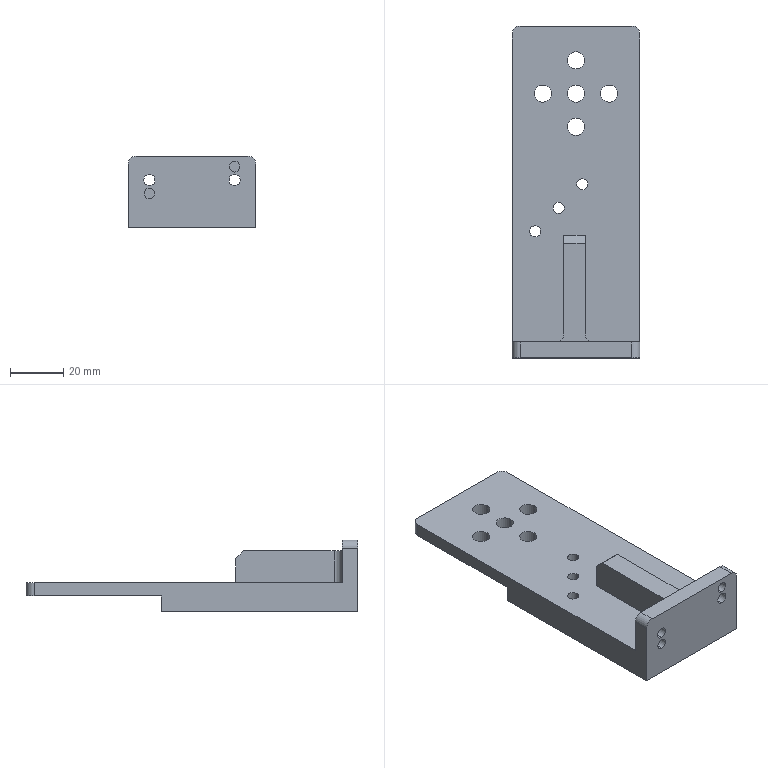NC program | NX | posted with a generic post | part box 48 x 124.7 x 27 mm
Whole program, first 1584 of 1777 lines:
N10 G17 G21 G94 G90
(FLOOR_WALL_COPY , TOOL : D80)
N12 T19 M6
N14 G54
N16 G17 G0 G90 X-111.35 Y0. B0. C0. S6500 M3
N18 G43 Z30. H19
N20 Z3.
N22 G94 G1 Z0. F1500.
N24 X-106.35
N26 X106.35
N28 X111.35
N30 Z3.
N32 G0 Z30.
N34 M5
(ADAPTIVE_MILLING , TOOL : D10)
N36 T15 M6
N38 G54
N40 G17 G0 G90 X-0.035 Y35.706 B0. C0. S9500 M3
N42 G43 Z30. H15
N44 Z-2.85
N46 G94 G1 Z-5.85 F1000.
N48 X-0.314 Y34.925 F3000.
N50 X-0.57 Y34.137
N52 G3 X-0.035 Y33.059 R1.017
N54 X3.029 Y32.298 R8.28
N56 X12.896 Y32.015 R111.643
N58 G1 X15.146 Y32.011
N60 X19.021 Y32.008
N62 X32.646 Y32.007
N64 X63.271
N66 X63.396 Y32.006
N68 X63.521 Y32.004
N70 G2 X67.796 Y29.5 R5.713
N72 X69.831 Y24.05 R12.236
N74 X70.306 Y15.57 R62.176
N76 G1 X70.315 Y14.446
N78 X70.323 Y13.071
N80 X70.329 Y11.196
N82 X70.333 Y8.446
N84 X70.335 Y3.071
N86 X70.336 Y-25.054
N88 G2 X67.993 Y-29.286 R5.635
N90 X62.588 Y-31.431 R11.953
N92 X54.988 Y-31.94 R51.981
N94 G1 X53.988 Y-31.953
N96 X52.988 Y-31.962
N98 X51.613 Y-31.971
N100 X49.863 Y-31.977
N102 X47.238 Y-31.982
N104 X42.613 Y-31.984
N106 X3.363 Y-31.985
N108 X-63.387
N110 X-63.512 Y-31.983
N112 X-63.637 Y-31.976
N114 X-63.762 Y-31.965
N116 G2 X-67.992 Y-29.146 R6.011
N118 X-69.896 Y-23.51 R13.346
N120 X-70.314 Y-14.526 R75.467
N122 G1 X-70.322 Y-13.151
N124 X-70.329 Y-11.276
N126 X-70.333 Y-8.651
N128 X-70.335 Y-3.651
N130 X-70.336 Y24.974
N132 X-70.335 Y25.099
N134 G2 X-67.854 Y29.389 R5.736
N136 X-62.294 Y31.479 R12.387
N138 X-53.814 Y31.955 R61.959
N140 G1 X-52.689 Y31.964
N142 X-51.314 Y31.972
N144 X-49.439 Y31.978
N146 X-46.689 Y31.983
N148 X-41.314 Y31.985
N150 X-3.814
N152 G2 X1.658 Y31.464 R60.908
N154 G3 X13.521 Y31.035 R127.721
N156 G1 X15.146 Y31.028
N158 X17.521 Y31.023
N160 X21.146 Y31.019
N162 X29.521 Y31.018
N164 X60.271 Y31.017
N166 X60.521 Y31.013
N168 G2 X66.702 Y27.322 R7.626
N170 X68.839 Y20.846 R15.66
N172 X69.3 Y10.988 R84.585
N174 G1 X69.309 Y9.613
N176 X69.316 Y7.863
N178 X69.321 Y5.363
N180 X69.324 Y1.238
N182 X69.325 Y-12.137
N184 Y-21.887
N186 G2 X65.75 Y-28.259 R7.595
N188 X59.299 Y-30.464 R15.393
N190 X49.942 Y-30.943 R76.184
N192 G1 X48.693 Y-30.953
N194 X47.193 Y-30.961
N196 X45.193 Y-30.967
N198 X42.318 Y-30.972
N200 X36.818 Y-30.974
N202 X-60.182
N204 X-60.432 Y-30.972
N206 X-60.682 Y-30.963
N208 X-60.807 Y-30.955
N210 G2 X-66.715 Y-27.232 R7.692
N212 X-68.841 Y-20.752 R15.777
N214 X-69.3 Y-10.893 R83.753
N216 G1 X-69.309 Y-9.519
N218 X-69.316 Y-7.769
N220 X-69.321 Y-5.269
N222 X-69.324 Y-1.269
N224 X-69.325 Y11.606
N226 Y21.856
N228 G2 X-65.669 Y28.31 R7.607
N230 X-59.079 Y30.493 R15.728
N232 X-49.971 Y30.943 R78.281
N234 G1 X-48.846 Y30.952
N236 X-47.471 Y30.96
N238 X-45.596 Y30.966
N240 X-42.846 Y30.971
N242 X-37.971 Y30.974
N244 X-6.221
N246 G2 X1.386 Y30.485 R99.342
N248 G3 X16.375 Y30.042 R194.129
N250 G1 X18.75 Y30.035
N252 X22.125 Y30.031
N254 X28.375 Y30.029
N256 X57.25 Y30.028
N258 X57.75 Y30.026
N260 X57.875 Y30.024
N262 G2 X65.811 Y25.229 R8.947
N264 X67.86 Y18.194 R18.674
N266 X68.285 Y8.458 R94.495
N268 G1 X68.294 Y7.083
N270 X68.302 Y5.333
N272 X68.309 Y2.833
N274 X68.312 Y-0.542
N276 X68.314 Y-8.042
N278 Y-19.292
N280 G2 X63.502 Y-27.467 R8.952
N282 X56.466 Y-29.51 R18.542
N284 X44.98 Y-29.945 R112.673
N286 G1 X43.105 Y-29.953
N288 X40.73 Y-29.958
N290 X36.855 Y-29.962
N292 X27.605 Y-29.964
N294 X-57.645
N296 X-57.895 Y-29.961
N298 G2 X-61.662 Y-29.177 R9.459
N300 X-63.747 Y-28.948 R16.345
N302 X-66.837 Y-26.511 R5.458
N304 X-67.495 Y-24.034 R5.984
N306 X-68.289 Y-8.94 R124.153
N308 G1 X-68.297 Y-7.44
N310 X-68.304 Y-5.565
N312 X-68.309 Y-2.94
N314 X-68.313 Y1.06
N316 X-68.314 Y11.185
N318 Y19.31
N320 G2 X-67.526 Y23.327 R9.637
N322 X-67.298 Y25.397 R15.666
N324 X-64.861 Y28.487 R5.458
N326 X-62.384 Y29.145 R5.984
N328 X-47.79 Y29.934 R121.449
N330 G1 X-46.29 Y29.944
N332 X-44.415 Y29.952
N334 X-42.04 Y29.957
N336 X-38.415 Y29.961
N338 X-30.915 Y29.963
N340 X-7.915 Y29.964
N342 G2 X0.822 Y29.518 R127.25
N344 G3 X12.709 Y29.114 R215.245
N346 X27.959 Y29.04 R784.32
N348 G1 X43.084 Y29.039
N350 X54.334
N352 X55.084 Y29.034
N354 X55.584 Y29.029
N356 X55.834 Y29.024
N358 X56.083 Y29.016
N360 G2 X64.76 Y23.61 R9.841
N362 X66.811 Y16.443 R19.883
N364 X67.27 Y6.208 R98.656
N366 G1 X67.281 Y4.833
N368 X67.289 Y3.208
N370 X67.295 Y1.083
N372 X67.3 Y-1.792
N374 X67.303 Y-6.917
N376 X67.304 Y-16.917
N378 G2 X65.585 Y-23.196 R10.36
N380 X59.426 Y-27.465 R11.896
N382 X51.799 Y-28.717 R30.693
N384 X38.178 Y-28.947 R261.114
N386 G1 X34.428 Y-28.951
N388 X26.178 Y-28.953
N390 X13.053
N392 X12.928 Y-28.959
N394 X12.887 Y-28.964
N396 X12.814 Y-28.984
N398 X11.584 Y-29.145
N400 X11.515 Y-29.15
N402 X-61.86
N404 G2 X-64.98 Y-28.418 R6.001
N406 X-67.334 Y-25.264 R5.458
N408 G1 X-67.495 Y-24.034
N410 X-67.5 Y-23.965
N412 Y23.535
N414 G2 X-66.768 Y26.63 R5.985
N416 X-63.614 Y28.984 R5.458
N418 G1 X-62.384 Y29.145
N420 X-62.315 Y29.15
N422 X11.515
N424 X11.584 Y29.145
N426 G2 X13.901 Y28.652 R9.504
N428 G3 X20.119 Y28.12 R34.015
N430 X35.869 Y28.05 R800.024
N432 G2 X54.493 Y28.002 R972.856
N434 X63.712 Y22.117 R10.517
N436 X65.769 Y14.819 R20.994
N438 X66.261 Y3.586 R105.233
N440 X66.256 Y-16.289 R937.524
N442 X60.371 Y-25.373 R10.478
N444 X53.193 Y-27.402 R21.037
N446 X41.71 Y-27.913 R104.229
N448 G1 X40.21 Y-27.922
N450 X38.335 Y-27.93
N452 X35.835 Y-27.936
N454 X32.085 Y-27.94
N456 X24.335 Y-27.942
N458 X16.085
N460 G3 X14.723 Y-28.044 R4.18
N462 G2 X12.827 Y-28.98 R6.626
N464 G3 X12.244 Y-30.51 R1.013
N466 G1 X12.605 Y-31.07
N468 X12.988 Y-31.616
N470 G3 X14.734 Y-30.901 R1.011
N472 G1 Z-2.85
N474 G0 Z30.
N476 X13.274 Y31.436
N478 Z-2.85
N480 G1 Z-5.85 F1000.
N482 G3 X11.457 Y30.806 R-1.01 F3000.
N484 G1 X12.729 Y29.125
N486 X12.887 Y28.999
N488 X13.063 Y28.9
N490 G3 X15.214 Y27.979 R69.717
N492 X20.897 Y27.212 R23.518
N494 X35.646 Y27.062 R427.881
N496 G2 X52.895 Y26.992 R751.352
N498 X62.736 Y20.577 R11.125
N500 X64.781 Y12.887 R22.827
N502 X65.251 Y1.526 R117.565
N504 X65.247 Y-14.473 R800.273
N506 X58.794 Y-24.409 R11.075
N508 X50.973 Y-26.45 R23.107
N510 X39.237 Y-26.904 R123.61
N512 G1 X37.612 Y-26.913
N514 X35.612 Y-26.92
N516 X32.612 Y-26.926
N518 X28.487 Y-26.93
N520 X18.987 Y-26.931
N522 X18.112 Y-26.937
N524 G3 X15.755 Y-27.138 R8.582
N526 X15.136 Y-27.684 R2.117
N528 G1 X14.541 Y-28.141
N530 G3 X14.489 Y-29.7 R1.013
N532 G1 X14.885 Y-30.052
N534 X15.294 Y-30.389
N536 G3 X16.836 Y-29.501 R1.012
N538 G1 Z-2.85
N540 G0 Z30.
N542 X15.049 Y30.779
N544 Z-2.85
N546 G1 Z-5.85 F1000.
N548 G3 X13.134 Y30.302 R-1.01 F3000.
N550 G1 X13.54 Y29.465
N552 X13.968 Y28.639
N554 X14.18 Y28.418
N556 G3 X17.78 Y26.79 R7.326
N558 X25.618 Y26.149 R46.049
N560 X45.743 Y26.069 R974.003
N562 G2 X52.363 Y25.901 R79.379
N564 X61.578 Y19.463 R11.462
N566 X63.735 Y11.546 R22.992
N568 X64.235 Y0.063 R114.775
N570 X64.22 Y-13.062 R417.223
N572 X57.455 Y-23.362 R11.529
N574 X49.509 Y-25.42 R23.817
N576 X37.274 Y-25.893 R127.791
N578 G1 X35.899 Y-25.901
N580 X33.899 Y-25.909
N582 X31.149 Y-25.915
N584 X27.024 Y-25.919
N586 X22.024 Y-25.92
N588 X20.899 Y-25.927
N590 X19.649 Y-25.937
N592 X19.274 Y-25.943
N594 X19.149 Y-25.946
N596 G3 X16.317 Y-26.336 R8.21
N598 G1 X16.211 Y-26.401
N600 X16.112 Y-26.478
N602 X16.02 Y-26.563
N604 X15.996 Y-26.58
N606 X15.968 Y-26.63
N608 X15.359 Y-27.424
N610 G3 X15.286 Y-28.532 R1.01
N612 X16.044 Y-29.031 Z-5.803 R1.046
N614 G1 X17.082 Y-29.246 Z-5.75
N616 X19.154 Y-29.668
N618 X33.631 Y-29.674
N620 G3 X47.321 Y-28.765 R104.449
N622 G1 X49.901 Y-28.424
N624 X52.478 Y-28.063
N626 G3 X59.478 Y-25.702 R23.042
N628 X62.152 Y-24.032 R32.386
N630 X63.976 Y-22.197 R8.956
N632 X66.464 Y-17.488 R16.584
N634 X66.915 Y-15.424 R14.301
N636 X67.368 Y-11.085 R37.066
N638 X67.445 Y-6.096 R62.706
N640 G1 X67.07 Y8.277
N642 G3 X66.414 Y14.473 R39.88
N644 G1 X66.185 Y15.699
N646 X65.904 Y16.914
N648 G3 X64.777 Y19.798 R16.586
N650 X62.924 Y23.047 R22.
N652 X61.061 Y25.285 R29.178
N654 X59.448 Y26.546 R7.461
N656 X56.779 Y27.894 R27.167
N658 X54.264 Y28.577 R12.145
N660 X50.556 Y28.975 R22.955
N662 G1 X18.819 Y29.713
N664 X16.615 Y29.722
N666 X15.961 Y29.73 Z-5.783
N668 X15.308 Y29.713 Z-5.815
N670 G3 X14.717 Y29.379 Z-5.85 R1.038
N672 X14.492 Y28.548 R1.016
N674 X15.136 Y27.684 R1.295
N676 X17.835 Y26.169 R5.508
N678 X24.633 Y25.261 R29.771
N680 X42.381 Y25.083 R489.163
N682 G2 X50.503 Y24.933 R136.592
N684 X60.618 Y18.01 R11.9
N686 X62.729 Y9.949 R24.232
N688 X63.225 Y-1.91 R119.841
N690 X63.191 Y-11.784 R216.134
N692 X56.252 Y-22.275 R11.909
N694 X48.314 Y-24.367 R24.155
N696 X36.455 Y-24.876 R119.317
N698 G1 X34.955 Y-24.886
N700 X33.08 Y-24.894
N702 X30.705 Y-24.901
N704 X27.455 Y-24.906
N706 X24.955 Y-24.908
N708 X23.955 Y-24.915
N710 X23.205 Y-24.917
N712 X22.205 Y-24.923
N714 X21.33 Y-24.933
N716 X20.955 Y-24.938
N718 G3 X17.121 Y-25.38 R13.244
N720 X16.037 Y-26.511 R1.532
N722 G1 X15.974 Y-26.619
N724 G3 X15.97 Y-27.612 R1.014
N726 X16.696 Y-28.113 Z-5.805 R1.05
N728 G1 X17.753 Y-28.375 Z-5.75
N730 X19.75 Y-28.862
N732 X24.888 Y-28.873
N734 X30.025 Y-28.854
N736 G3 X44.191 Y-27.92 R140.231
N738 G1 X47.666 Y-27.517
N740 X51.139 Y-27.089
N742 G3 X57.523 Y-25.034 R21.966
N744 X62.06 Y-21.845 R15.427
N746 G1 X63.212 Y-20.641
N748 G3 X64.339 Y-18.926 R7.881
N750 X65.496 Y-16.169 R28.464
N752 X65.901 Y-14.227 R9.459
N754 X66.375 Y-8.003 R117.455
N756 G1 X66.512 Y-5.039
N758 X66.594 Y-2.073
N760 G3 X66.182 Y6.333 R74.972
N762 G1 X65.907 Y8.922
N764 X65.618 Y11.509
N766 G3 X64.747 Y15.568 R28.451
N768 G1 X64.394 Y16.765
N770 X63.997 Y17.95
N772 G3 X62.296 Y21.274 R16.442
N774 G1 X61.314 Y22.719
N776 G3 X57.949 Y25.628 R10.939
N778 X53.23 Y27.478 R14.704
N780 X50.274 Y27.879 R21.595
N782 G1 X19.131 Y29.836
N784 X18.861 Y29.817
N786 X16.97 Y29.417
N788 X16.314 Y29.283 Z-5.784
N790 X15.662 Y29.126 Z-5.817
N792 G3 X15.168 Y28.707 Z-5.85 R1.041
N794 X15.234 Y27.586 R1.01
N796 X18.221 Y25.446 R5.386
N798 X24.861 Y24.35 R26.004
N800 X39.482 Y24.098 R278.956
N802 G2 X48.854 Y23.949 R187.644
N804 X56.948 Y20.497 R12.355
N806 X60.906 Y13.091 R15.896
N808 X62.061 Y3.678 R46.236
N810 X62.172 Y-10.318 R212.705
N812 X58.773 Y-18.56 R12.342
N814 X51.623 Y-22.481 R15.607
N816 X42.72 Y-23.674 R42.357
N818 X25.098 Y-23.908 R462.336
N820 G3 X18.984 Y-24.169 R46.763
N822 X16.772 Y-24.956 R4.616
N824 X16.211 Y-26.09 R3.818
N826 X16.438 Y-27.19 R1.01
N828 X17.296 Y-27.464 Z-5.803 R1.047
N830 G1 X18.362 Y-27.395 Z-5.75
N832 X20.558 Y-27.255
N834 X36.808
N836 G3 X46.749 Y-26.495 R65.951
N838 G1 X50.575 Y-25.893
N840 G3 X57.678 Y-23.135 R20.586
N842 X60.422 Y-21.239 R29.156
N844 X62.956 Y-18.409 R13.153
N846 X64.481 Y-15.028 R10.236
N848 X65.036 Y-11.711 R25.141
N850 G1 X65.124 Y-10.592
N852 X65.171 Y-9.471
N854 X65.343 Y0.528
N856 G3 X64.752 Y9.227 R52.015
N858 G1 X64.246 Y12.435
N860 G3 X63.062 Y16.496 R20.997
N862 X61.92 Y18.704 R16.474
N864 G1 X60.264 Y21.343
N866 G3 X59.286 Y22.55 R7.279
N868 G1 X58.262 Y23.418
N870 X57.226 Y24.271
N872 G3 X54.4 Y25.83 R12.036
N874 X50.783 Y26.713 R12.454
N876 X42.684 Y27.242 R186.451
N878 G1 X19.95 Y28.163
N880 X17.747 Y28.446
N882 X17.095 Y28.535 Z-5.783
N884 X16.441 Y28.599 Z-5.816
N886 G3 X15.819 Y28.347 Z-5.85 R1.039
N888 X15.691 Y26.991 R1.005
N890 X17.102 Y25.471 R5.483
N892 X21.921 Y23.831 R12.773
N894 X31.89 Y23.172 R70.477
N896 G2 X46.888 Y22.988 R775.762
N898 X53.889 Y20.965 R13.899
N900 X59.182 Y14.034 R13.777
N902 X60.83 Y5.722 R31.255
N904 X61.135 Y-9.142 R141.978
N906 X57.546 Y-17.567 R12.593
N908 X50.368 Y-21.444 R16.016
N910 X41.341 Y-22.657 R42.942
N912 X24.72 Y-22.916 R482.485
N914 G3 X18.874 Y-23.372 R28.465
N916 X16.857 Y-24.309 R4.386
N918 X16.501 Y-25.385 R2.115
N920 X16.758 Y-26.348 R1.014
N922 X17.594 Y-26.64 Z-5.804 R1.049
N924 G1 X18.678 Y-26.61 Z-5.75
N926 X20.848 Y-26.549
N928 X30.223
N930 G3 X43.913 Y-25.641 R104.449
N932 G1 X46.7 Y-25.271
N934 X49.484 Y-24.887
N936 G3 X55.884 Y-22.536 R19.394
N938 X60.14 Y-19.304 R21.663
N940 X62.335 Y-16.003 R11.567
N942 G1 X63.337 Y-13.721
N944 G3 X63.827 Y-11.924 R6.864
N946 G1 X64.26 Y-7.753
N948 G3 X64.343 Y-1.346 R46.365
N950 G1 X64.108 Y2.814
N952 X63.852 Y6.972
N954 G3 X61.943 Y15.254 R32.188
N956 X59.611 Y19.643 R19.899
N958 X57.989 Y21.524 R15.572
N960 G1 X56.348 Y23.119
N962 G3 X53.266 Y24.853 R8.95
N964 X48.017 Y25.817 R23.24
N966 G1 X18.191 Y27.816
N968 X17.525 Y27.864 Z-5.783
N970 X16.859 Y27.888 Z-5.817
N972 G3 X16.266 Y27.613 Z-5.85 R1.04
N974 X16.037 Y26.511 R1.01
N976 X17.94 Y24.444 R3.889
N978 X23.412 Y22.786 R15.731
N980 X34.137 Y22.173 R85.721
N982 G2 X45.635 Y21.984 R484.936
N984 X52.646 Y19.977 R14.365
N986 X58.124 Y12.884 R13.949
N988 X59.82 Y4.328 R31.846
N990 X60.087 Y-8.036 R103.638
N992 X56.099 Y-16.795 R12.688
N994 X48.578 Y-20.56 R16.926
N996 X39.159 Y-21.679 R49.273
N998 X24.287 Y-21.938 R840.384
N1000 G3 X18.721 Y-22.625 R21.206
N1002 X16.825 Y-23.767 R3.615
N1004 X16.587 Y-24.857 R3.059
N1006 X16.955 Y-25.769 R1.014
N1008 X17.759 Y-25.99 Z-5.807 R1.173
N1010 G1 X18.905 Y-26.001 Z-5.75
N1012 X21.481 Y-26.012
N1014 X24.056 Y-25.965
N1016 G3 X30.289 Y-25.626 R89.658
N1018 G1 X44.607 Y-24.324
N1020 G3 X54.182 Y-21.719 R28.478
N1022 G1 X55.268 Y-21.206
N1024 X56.347 Y-20.677
N1026 G3 X59.221 Y-18.24 R9.631
N1028 X61.246 Y-15.105 R17.5
N1030 X62.769 Y-10.433 R14.094
N1032 X63.158 Y-5.465 R42.479
N1034 G1 X63.232 Y-0.604
N1036 G3 X62.425 Y8.208 R51.287
N1038 G1 X62.095 Y10.052
N1040 X61.747 Y11.893
N1042 G3 X60.067 Y16.16 R15.692
N1044 X58.85 Y18.041 R20.831
N1046 G1 X58.124 Y19.026
N1048 X57.362 Y19.983
N1050 G3 X55.375 Y21.853 R11.039
N1052 G1 X54.957 Y22.122
N1054 X54.529 Y22.373
N1056 X53.433 Y22.962
N1058 X52.316 Y23.512
N1060 G3 X49.252 Y24.485 R12.582
N1062 X38.826 Y25.648 R274.358
N1064 G1 X20.499 Y27.331
N1066 X18.358 Y27.468
N1068 X17.683 Y27.516 Z-5.784
N1070 X17.007 Y27.542 Z-5.818
N1072 G3 X16.427 Y27.283 Z-5.85 R1.042
N1074 X16.18 Y26.164 R1.01
N1076 X18.53 Y23.533 R4.519
N1078 X24.498 Y21.793 R17.436
N1080 X34.849 Y21.191 R89.248
N1082 G2 X44.845 Y20.951 R222.906
N1084 X52.406 Y18.316 R13.844
N1086 X57.312 Y11.077 R14.956
N1088 X58.873 Y2.112 R36.215
N1090 X59.014 Y-7.13 R69.228
N1092 X51.673 Y-17.98 R12.801
N1094 X43.145 Y-20.266 R25.644
N1096 X32.163 Y-20.812 R109.366
N1098 G3 X22.793 Y-21.065 R174.236
N1100 X18.065 Y-22.132 R13.322
N1102 X16.77 Y-23.256 R2.532
N1104 X16.679 Y-24.158 R4.534
N1106 X17.078 Y-25.094 R1.011
N1108 X17.856 Y-25.291 Z-5.809 R1.199
N1110 G1 X19.036 Y-25.304 Z-5.75
N1112 X21.026 Y-25.323
N1114 X38.474 Y-23.981
N1116 G3 X45.889 Y-22.952 R62.285
N1118 G1 X48.337 Y-22.447
N1120 G3 X52.128 Y-21.068 R18.9
N1122 X56.196 Y-18.768 R41.277
N1124 X57.41 Y-17.8 R6.639
N1126 X59.153 Y-15.603 R30.304
N1128 X61.526 Y-9.926 R14.502
N1130 G1 X61.836 Y-8.185
N1132 X62.106 Y-6.437
N1134 G3 X62.245 Y-3.119 R16.457
N1136 G1 X61.98 Y0.829
N1138 X61.69 Y4.776
N1140 G3 X60.831 Y9.896 R38.241
N1142 G1 X60.54 Y11.108
N1144 X60.195 Y12.306
N1146 G3 X58.429 Y15.853 R16.02
N1148 X56.345 Y18.647 R32.723
N1150 X49.749 Y23.07 R13.028
N1152 X46.702 Y23.69 R18.346
N1154 G1 X20.765 Y26.64
N1156 X18.653 Y26.775
N1158 X17.975 Y26.823 Z-5.784
N1160 X17.295 Y26.849 Z-5.818
N1162 G3 X16.72 Y26.595 Z-5.85 R1.043
N1164 X16.467 Y25.471 R1.007
N1166 X18.193 Y23.151 R3.804
N1168 X23.531 Y21.126 R14.162
N1170 X32.983 Y20.274 R60.021
N1172 G2 X43.353 Y19.978 R340.49
N1174 X50.774 Y17.648 R14.664
N1176 X56.142 Y10.304 R14.643
N1178 X57.797 Y1.611 R33.954
N1180 X57.879 Y-6.626 R44.639
N1182 X50.631 Y-16.883 R12.833
N1184 X42.613 Y-19.161 R24.921
N1186 X30.637 Y-19.812 R110.188
N1188 G3 X22.151 Y-20.223 R85.513
N1190 X17.76 Y-21.561 R11.098
N1192 X16.717 Y-22.75 R2.044
N1194 G1 X16.7 Y-22.872
N1196 Y-23.622
N1198 G3 X17.252 Y-24.516 R1.011
N1200 X18.18 Y-24.52 Z-5.802 R1.139
N1202 G1 X19.174 Y-24.209 Z-5.75
N1204 X20.108 Y-23.91
N1206 X21.049 Y-23.634
N1208 X21.2 Y-23.622
N1210 X27.627 Y-23.61
N1212 G3 X36.161 Y-23.002 R81.628
N1214 G1 X40.295 Y-22.49
N1216 X44.427 Y-21.957
N1218 G3 X53.607 Y-18.807 R27.116
N1220 X56.917 Y-16.05 R13.601
N1222 X60.261 Y-10.152 R14.873
N1224 X61.2 Y-3.738 R23.335
N1226 G1 Y-1.703
N1228 X61.143 Y0.33
N1230 G3 X59.441 Y9.938 R42.347
N1232 X57.462 Y14.485 R22.102
N1234 G1 X56.202 Y16.638
N1236 G3 X55.043 Y18.098 R7.28
N1238 X52.082 Y20.381 R15.814
N1240 X47.281 Y22.342 R15.328
N1242 X45.076 Y22.712 R20.646
N1244 G1 X20.921 Y25.282
N1246 X18.953 Y25.958
N1248 X18.326 Y26.181 Z-5.783
N1250 X17.691 Y26.381 Z-5.817
N1252 G3 X17.044 Y26.271 Z-5.85 R1.04
N1254 X16.534 Y25.264 R1.01
N1256 X17.868 Y22.813 R3.412
N1258 X22.438 Y20.586 R11.634
N1260 X31.466 Y19.39 R42.69
N1262 G2 X41.958 Y19.008 R855.284
N1264 X48.994 Y17.04 R15.649
N1266 X54.871 Y9.8 R14.315
N1268 X56.712 Y1.149 R31.295
N1270 X56.653 Y-6.455 R29.907
N1272 X49.619 Y-15.777 R12.854
N1274 X41.246 Y-18.157 R25.048
N1276 X32.019 Y-18.75 R94.343
N1278 G3 X23.157 Y-19.187 R108.754
N1280 X18.127 Y-20.573 R13.783
N1282 X16.771 Y-21.823 R3.031
N1284 X16.7 Y-22.997 R4.011
N1286 X17.264 Y-23.897 R1.011
N1288 X18.176 Y-23.897 Z-5.803 R1.149
N1290 G1 X19.19 Y-23.588 Z-5.75
N1292 X21.094 Y-23.012
N1294 X39.262 Y-21.492
N1296 G3 X45.418 Y-20.514 R42.568
N1298 G1 X46.632 Y-20.227
N1300 X47.834 Y-19.893
N1302 G3 X51.441 Y-18.236 R17.985
N1304 G1 X52.391 Y-17.642
N1306 X53.315 Y-17.009
N1308 X54.275 Y-16.315
N1310 X55.225 Y-15.606
N1312 G3 X57.152 Y-13.35 R8.994
N1314 X58.105 Y-11.464 R14.871
N1316 X59.781 Y-5.748 R23.1
N1318 X59.992 Y-0.534 R19.419
N1320 G1 X59.576 Y3.401
N1322 G3 X56.907 Y12.769 R33.913
N1324 X54.466 Y16.358 R12.938
N1326 G1 X52.771 Y18.069
N1328 G3 X50.158 Y19.852 R10.924
N1330 X46.696 Y21.233 R19.72
N1332 G1 X45.79 Y21.446
N1334 X44.872 Y21.604
N1336 X21.001 Y24.786
N1338 X19.041 Y25.456
N1340 X18.404 Y25.681 Z-5.784
N1342 X17.759 Y25.884 Z-5.818
N1344 G3 X17.13 Y25.787 Z-5.85 R1.042
N1346 X16.599 Y24.768 R1.007
N1348 X18.1 Y21.998 R3.773
N1350 X23.017 Y19.633 R12.605
N1352 X32.419 Y18.402 R45.593
N1354 G2 X41.283 Y17.985 R254.256
N1356 X48.973 Y15.303 R14.933
N1358 X54.078 Y8.052 R15.209
N1360 X55.671 Y-4.387 R31.712
N1362 X48.522 Y-14.715 R12.853
N1364 X40.157 Y-17.124 R24.935
N1366 X29.933 Y-17.789 R109.912
N1368 G3 X22.092 Y-18.443 R58.951
N1370 X17.571 Y-20.157 R10.962
N1372 X16.7 Y-21.354 R1.854
N1374 G1 Y-22.229
N1376 G3 X17.264 Y-23.129 R1.011
N1378 X18.176 Y-23.13 Z-5.803 R1.149
N1380 G1 X19.19 Y-22.821 Z-5.75
N1382 X21.098 Y-22.244
N1384 X36.138 Y-20.871
N1386 G3 X45.848 Y-19.056 R53.573
N1388 X51.082 Y-17.016 R35.109
N1390 X55.002 Y-13.829 R12.152
N1392 X57.573 Y-9.695 R18.953
N1394 X58.895 Y-3.76 R13.232
N1396 X58.479 Y2.67 R47.049
N1398 X57.69 Y6.749 R35.547
N1400 X54.722 Y13.517 R24.012
N1402 G1 X54.129 Y14.439
N1404 X53.499 Y15.336
N1406 G3 X50.56 Y17.99 R10.835
N1408 X46.086 Y20.127 R20.505
N1410 X41.29 Y21.315 R24.469
N1412 G1 X21.086 Y24.166
N1414 X19.131 Y24.834
N1416 X18.49 Y25.06 Z-5.784
N1418 X17.842 Y25.264 Z-5.818
N1420 G3 X17.22 Y25.171 Z-5.85 R1.043
N1422 X16.68 Y24.148 R1.007
N1424 X17.876 Y21.564 R3.486
N1426 X22.651 Y18.942 R11.633
N1428 X31.393 Y17.53 R38.723
N1430 G2 X40.376 Y16.989 R284.794
N1432 X48.019 Y14.18 R14.902
N1434 X53.11 Y6.766 R15.534
N1436 X54.475 Y-3.57 R25.362
N1438 X47.619 Y-13.552 R12.681
N1440 X39.534 Y-16.025 R24.039
N1442 X30.067 Y-16.763 R99.057
N1444 G3 X21.99 Y-17.573 R55.47
N1446 X17.516 Y-19.406 R11.093
N1448 X16.7 Y-20.581 R1.833
N1450 G1 Y-21.456
N1452 G3 X17.263 Y-22.356 R1.011
N1454 X18.176 Y-22.357 Z-5.803 R1.149
N1456 G1 X19.189 Y-22.048 Z-5.75
N1458 X21.103 Y-21.471
N1460 X33.016 Y-20.274
N1462 G3 X41.619 Y-18.8 R63.069
N1464 G1 X44.771 Y-18.016
N1466 G3 X50.226 Y-15.613 R20.389
N1468 G1 X51.478 Y-14.755
N1470 X52.717 Y-13.877
N1472 G3 X54.532 Y-11.908 R8.713
N1474 X56.699 Y-7.443 R17.807
N1476 X57.367 Y-4.41 R25.456
N1478 X57.736 Y-1.318 R24.961
N1480 X57.516 Y1.78 R16.105
N1482 X55.707 Y8.639 R31.676
N1484 X52.287 Y14.255 R20.161
N1486 X45.881 Y18.877 R15.31
N1488 X43.651 Y19.493 R14.436
N1490 G1 X21.098 Y23.74
N1492 X19.202 Y24.309
N1494 X18.526 Y24.514 Z-5.785
N1496 X17.845 Y24.705 Z-5.821
N1498 G3 X17.274 Y24.62 Z-5.85 R1.051
N1500 X16.7 Y23.715 R1.011
N1502 X17.857 Y20.92 R3.565
N1504 X22.562 Y18.173 R11.617
N1506 X31.4 Y16.598 R37.157
N1508 G2 X39.378 Y16.011 R215.884
N1510 X46.995 Y13.123 R15.131
N1512 X52.069 Y5.695 R15.68
N1514 X53.171 Y-3.16 R19.759
N1516 X46.768 Y-12.352 R12.434
N1518 X38.602 Y-14.972 R23.57
N1520 X29.017 Y-15.811 R115.839
N1522 G3 X21.348 Y-16.846 R42.036
N1524 X17.23 Y-18.852 R9.688
N1526 X16.7 Y-19.778 R1.515
N1528 G1 Y-20.653
N1530 G3 X17.263 Y-21.553 R1.011
N1532 X18.175 Y-21.554 Z-5.803 R1.15
N1534 G1 X19.189 Y-21.246 Z-5.75
N1536 X21.11 Y-20.668
N1538 X26.785 Y-20.009
N1540 X29.567 Y-19.613
N1542 X32.341 Y-19.158
N1544 X40.958 Y-17.629
N1546 G3 X47.442 Y-15.494 R24.876
N1548 X50.276 Y-13.594 R16.538
N1550 X52.769 Y-11.375 R32.077
N1552 X54.6 Y-8.787 R10.865
N1554 G1 X55.145 Y-7.707
N1556 X55.675 Y-6.62
N1558 G3 X56.504 Y-2.381 R10.019
N1560 X55.56 Y4.654 R34.338
N1562 X52.155 Y12.099 R23.104
N1564 X49.751 Y14.796 R14.747
N1566 X45.219 Y17.557 R19.29
N1568 G1 X44.347 Y17.881
N1570 X43.456 Y18.151
N1572 G3 X37.393 Y19.637 R155.823
N1574 G1 X21.129 Y23.234
N1576 X19.221 Y23.804
N1578 X17.848 Y24.204 Z-5.822
N1580 G3 X17.292 Y24.128 Z-5.85 R1.054
N1582 X16.7 Y23.215 R1.01
N1584 X17.819 Y20.272 R3.744
N1586 X22.454 Y17.41 R11.544
N1588 X31.262 Y15.686 R35.044
N1590 G2 X39.099 Y14.937 R116.957
N1592 X48.406 Y9.611 R14.182
N1594 X51.891 Y-1.988 R17.213
N1596 X45.99 Y-11.08 R11.981
N1598 X38.012 Y-13.859 R22.133
N1600 X28.566 Y-14.84 R121.77
N1602 G3 X20.933 Y-16.089 R36.889
N1604 X17.118 Y-18.144 R9.172
N1606 X16.7 Y-18.954 R1.433
N1608 G1 Y-19.829
N1610 G3 X17.263 Y-20.728 R1.011
N1612 X18.174 Y-20.73 Z-5.803 R1.15
N1614 G1 X19.189 Y-20.423 Z-5.75
N1616 X21.037 Y-19.863
N1618 X21.2 Y-19.829
N1620 X24.297 Y-19.431
N1622 X27.387 Y-18.982
N1624 X28.925 Y-18.714
N1626 X30.46 Y-18.429
N1628 X40.272 Y-16.492
N1630 G3 X45.253 Y-14.911 R22.781
N1632 X49.277 Y-12.448 R22.159
N1634 X52.566 Y-8.988 R18.353
N1636 X54.07 Y-5.961 R11.878
N1638 X54.805 Y-3.073 R19.016
N1640 G1 X55.089 Y-1.309
N1642 G3 X54.94 Y1.842 R9.99
N1644 X53.787 Y6.048 R36.191
N1646 X52.43 Y8.839 R15.394
N1648 G1 X51.498 Y10.339
N1650 X50.527 Y11.814
N1652 X50.041 Y12.485
N1654 X49.513 Y13.124
N1656 G3 X48.265 Y14.2 R7.825
N1658 G1 X47.239 Y14.904
N1660 X46.188 Y15.57
N1662 G3 X42.777 Y17.035 R14.021
N1664 X31.3 Y20.061 R568.799
N1666 G1 X21.157 Y22.602
N1668 X19.221 Y23.18
N1670 X17.847 Y23.579 Z-5.822
N1672 G3 X17.291 Y23.503 Z-5.85 R1.054
N1674 X16.7 Y22.59 R1.01
N1676 X17.848 Y19.528 R3.885
N1678 X22.681 Y16.516 R12.014
N1680 X30.981 Y14.79 R34.885
N1682 G2 X38.428 Y13.918 R92.657
N1684 X49.708 Y4.224 R14.428
N1686 X49.639 Y-4.567 R12.082
N1688 X43.306 Y-10.864 R12.761
N1690 X35.27 Y-13.094 R26.814
N1692 G1 X34.898 Y-13.146
N1694 X34.403 Y-13.21
N1696 X34.03 Y-13.256
N1698 X33.534 Y-13.315
N1700 X32.913 Y-13.384
N1702 X32.291 Y-13.451
N1704 X31.421 Y-13.539
N1706 X29.804 Y-13.699
N1708 X28.933 Y-13.789
N1710 X27.939 Y-13.896
N1712 X27.318 Y-13.965
N1714 X26.697 Y-14.039
N1716 X26.573 Y-14.054
N1718 X26.078 Y-14.12
N1720 X25.706 Y-14.172
N1722 G3 X19.319 Y-15.841 R23.074
N1724 X16.836 Y-17.678 R5.946
N1726 X16.7 Y-19.005 R2.911
N1728 X17.262 Y-19.904 R1.011
N1730 X18.173 Y-19.907 Z-5.803 R1.15
N1732 G1 X19.189 Y-19.601 Z-5.75
N1734 X21.2 Y-19.005
N1736 G3 X30.409 Y-17.293 R271.31
N1738 G1 X40.201 Y-15.254
N1740 G3 X45.401 Y-13.247 R16.747
N1742 G1 X46.18 Y-12.734
N1744 X46.929 Y-12.179
N1746 X48.863 Y-10.616
N1748 G3 X51.654 Y-7.324 R14.553
N1750 G1 X52.515 Y-5.903
N1752 G3 X53.318 Y-3.356 R7.751
N1754 G1 X53.429 Y-2.428
N1756 X53.489 Y-1.495
N1758 X53.544 Y0.913
N1760 G3 X53.016 Y4.033 R10.994
N1762 X51.682 Y7.526 R27.703
N1764 X48.454 Y12.085 R19.115
N1766 X44.971 Y14.644 R12.534
N1768 X39.773 Y16.687 R27.912
N1770 G1 X21.182 Y21.846
N1772 X19.22 Y22.431
N1774 X17.847 Y22.829 Z-5.822
N1776 G3 X17.29 Y22.752 Z-5.85 R1.054
N1778 X16.7 Y21.84 R1.01
N1780 X17.865 Y18.779 R4.004
N1782 X22.661 Y15.706 R12.223
N1784 X31.062 Y13.853 R34.746
N1786 G2 X38.107 Y12.818 R60.642
N1788 X48.747 Y2.214 R13.889
N1790 X44.801 Y-8.094 R10.492
N1792 X37.232 Y-11.507 R18.553
N1794 X28.707 Y-12.79 R82.805
N1796 G3 X20.873 Y-14.339 R39.743
N1798 X17.192 Y-16.394 R9.764
N1800 X16.7 Y-17.283 R1.524
N1802 G1 Y-18.158
N1804 G3 X17.262 Y-19.057 R1.011
N1806 X18.172 Y-19.061 Z-5.803 R1.151
N1808 G1 X19.189 Y-18.756 Z-5.75
N1810 X21.2 Y-18.158
N1812 X32.232 Y-15.952
N1814 G3 X41.349 Y-13.479 R73.851
N1816 X45.212 Y-11.681 R22.554
N1818 G1 X46.64 Y-10.828
N1820 G3 X48.588 Y-8.993 R8.451
N1822 X51.054 Y-4.684 R17.738
N1824 G1 X51.259 Y-4.098
N1826 X51.448 Y-3.506
N1828 X51.764 Y-2.408
N1830 X52.065 Y-1.305
N1832 G3 X52.17 Y0.74 R6.473
N1834 X51.516 Y3.786 R17.228
N1836 X50.101 Y7.233 R16.903
N1838 G1 X48.948 Y9.305
N1840 G3 X46.611 Y11.863 R10.204
N1842 X43.711 Y13.794 R30.036
N1844 X39.689 Y15.395 R17.204
N1846 G1 X36.679 Y16.22
N1848 X33.655 Y16.991
N1850 X21.047 Y20.051
N1852 X20.857 Y20.122
N1854 X20.681 Y20.223
N1856 X19.218 Y21.324
N1858 X18.695 Y21.724 Z-5.783
N1860 X18.157 Y22.105 Z-5.816
N1862 G3 X17.494 Y22.194 Z-5.85 R1.039
N1864 X16.7 Y21.215 R1.007
N1866 X17.951 Y17.933 R4.193
N1868 X22.978 Y14.758 R12.863
N1870 X30.756 Y12.963 R35.909
N1872 G2 X37.641 Y11.737 R50.144
N1874 X46.083 Y5.161 R13.583
N1876 X43.968 Y-6.583 R9.617
N1878 X37.308 Y-10.149 R16.307
N1880 X29.085 Y-11.697 R58.675
N1882 G3 X21.379 Y-13.269 R47.246
N1884 X17.318 Y-15.411 R11.119
N1886 X16.7 Y-16.43 R1.671
N1888 G1 Y-17.305
N1890 G3 X17.261 Y-18.204 R1.011
N1892 X18.171 Y-18.208 Z-5.803 R1.151
N1894 G1 X19.189 Y-17.903 Z-5.75
N1896 X21.2 Y-17.305
N1898 X30.962 Y-15.136
N1900 G3 X40.012 Y-12.427 R69.007
N1902 X43.772 Y-10.453 R19.507
N1904 G1 X45.832 Y-9.046
N1906 G3 X46.997 Y-8.019 R6.63
N1908 G1 X47.798 Y-6.943
N1910 X48.581 Y-5.855
N1912 G3 X50.148 Y-1.696 R10.517
N1914 X50.335 Y1.569 R12.887
N1916 X49.01 Y6.133 R12.259
N1918 G1 X48.524 Y7.071
N1920 X47.997 Y7.987
N1922 G3 X45.425 Y10.903 R13.168
N1924 X40.084 Y14.018 R17.654
N1926 X36.521 Y15.152 R42.579
N1928 G1 X21.047 Y19.301
N1930 X20.871 Y19.371
N1932 X20.707 Y19.466
N1934 X19.218 Y20.579
N1936 X18.693 Y20.978 Z-5.783
N1938 X18.154 Y21.356 Z-5.816
N1940 G3 X17.491 Y21.443 Z-5.85 R1.039
N1942 X16.7 Y20.465 R1.007
N1944 X17.865 Y17.273 R4.177
N1946 X22.818 Y13.988 R12.638
N1948 X30.563 Y12.055 R36.046
N1950 G2 X37.038 Y10.687 R42.201
N1952 X43.839 Y5.842 R13.062
N1954 X43.16 Y-4.801 R8.628
N1956 X36.82 Y-8.875 R14.439
N1958 X29.151 Y-10.62 R46.98
N1960 G3 X21.471 Y-12.324 R52.82
N1962 X17.311 Y-14.546 R11.543
N1964 X16.7 Y-15.56 R1.676
N1966 G1 Y-16.435
N1968 G3 X17.261 Y-17.333 R1.011
N1970 X18.171 Y-17.338 Z-5.803 R1.151
N1972 G1 X19.189 Y-17.034 Z-5.75
N1974 X21.2 Y-16.435
N1976 X30.901 Y-14.01
N1978 G3 X39.226 Y-11.178 R54.085
N1980 X43.852 Y-8.235 R19.283
N1982 G1 X45.189 Y-7.065
N1984 G3 X48.014 Y-2.059 R10.278
N1986 G1 X48.121 Y-1.541
N1988 X48.212 Y-1.02
N1990 X48.458 Y0.834
N1992 X48.497 Y1.454
N1994 X48.478 Y2.076
N1996 X48.36 Y2.684
N1998 X47.713 Y4.965
N2000 G3 X46.187 Y7.802 R10.521
N2002 X43.864 Y10.366 R17.244
N2004 X41.492 Y11.964 R12.832
N2006 X38.172 Y13.375 R21.684
N2008 G1 X35.805 Y14.17
N2010 X33.421 Y14.91
N2012 X20.936 Y18.59
N2014 X20.732 Y18.707
N2016 X19.218 Y19.833
N2018 X18.692 Y20.23 Z-5.783
N2020 X18.152 Y20.607 Z-5.816
N2022 G3 X17.489 Y20.693 Z-5.85 R1.039
N2024 X16.7 Y19.715 R1.007
N2026 X17.932 Y16.42 R4.302
N2028 X23.114 Y13.032 R13.221
N2030 X30.851 Y11.049 R41.197
N2032 G2 X37.456 Y9.206 R28.406
N2034 X42.392 Y4.957 R10.407
N2036 X41.547 Y-3.616 R7.829
N2038 X35.703 Y-7.752 R13.252
N2040 X29.073 Y-9.534 R40.062
N2042 G3 X21.314 Y-11.455 R57.554
N2044 X17.209 Y-13.773 R11.248
N2046 X16.7 Y-14.685 R1.572
N2048 G1 Y-15.56
N2050 G3 X17.261 Y-16.459 R1.011
N2052 X18.171 Y-16.463 Z-5.803 R1.151
N2054 G1 X19.189 Y-16.16 Z-5.75
N2056 X21.2 Y-15.56
N2058 X34.927 Y-11.292
N2060 G3 X41.089 Y-8.508 R27.479
N2062 X44.9 Y-4.535 R11.933
N2064 X46.005 Y-2.221 R10.484
N2066 X46.402 Y0.659 R8.785
N2068 X45.516 Y5.524 R13.811
N2070 X43.731 Y8.475 R8.379
N2072 X40.404 Y11.081 R14.488
N2074 G1 X39.692 Y11.438
N2076 X38.96 Y11.752
N2078 G3 X31.911 Y14.281 R128.913
N2080 G1 X21.047 Y17.801
N2082 X20.9 Y17.867
N2084 X20.761 Y17.948
N2086 X19.22 Y19.086
N2088 X18.692 Y19.482 Z-5.783
N2090 X18.15 Y19.858 Z-5.816
N2092 G3 X17.488 Y19.943 Z-5.85 R1.039
N2094 X16.7 Y18.965 R1.007
N2096 X17.91 Y15.658 R4.352
N2098 X22.938 Y12.258 R13.165
N2100 X29.9 Y10.276 R39.384
N2102 G2 X36.234 Y8.383 R29.743
N2104 X40.324 Y4.684 R8.274
N2106 X39.535 Y-2.655 R7.201
N2108 X34.015 Y-6.809 R12.552
N2110 X27.193 Y-8.832 R44.13
N2112 G3 X20.266 Y-10.942 R42.609
N2114 X16.975 Y-13.154 R8.911
N2116 X16.7 Y-13.805 R1.467
N2118 G1 Y-14.805
N2120 G3 X17.261 Y-15.703 R1.011
N2122 X18.171 Y-15.708 Z-5.803 R1.151
N2124 G1 X19.189 Y-15.405 Z-5.75
N2126 X21.2 Y-14.805
N2128 X32.994 Y-10.662
N2130 G3 X38.915 Y-7.634 R25.156
N2132 X41.358 Y-5.276 R12.977
N2134 X43.046 Y-2.813 R19.201
N2136 G1 X43.855 Y-1.372
N2138 G3 X44.384 Y1.761 R5.754
N2140 X43.397 Y5.333 R12.166
N2142 G1 X42.929 Y6.375
N2144 X42.443 Y7.409
N2146 G3 X40.777 Y9.308 R5.934
N2148 X39.071 Y10.315 R8.73
N2150 X31.557 Y13.36 R96.596
N2152 G1 X21.047 Y17.051
N2154 X20.786 Y17.188
N2156 X19.217 Y18.341
N2158 X18.689 Y18.736 Z-5.783
N2160 X18.147 Y19.11 Z-5.816
N2162 G3 X17.483 Y19.191 Z-5.85 R1.039
N2164 X16.7 Y18.215 R1.007
N2166 X17.88 Y14.895 R4.4
N2168 X22.871 Y11.439 R13.274
N2170 X29.432 Y9.416 R41.307
N2172 G2 X34.77 Y7.676 R27.66
N2174 X37.806 Y-0.652 R6.199
N2176 X33.378 Y-5.258 R10.172
N2178 X27.342 Y-7.626 R28.055
N2180 G3 X20.239 Y-10.013 R53.92
N2182 X16.97 Y-12.262 R9.063
N2184 X16.7 Y-12.905 R1.49
N2186 G1 Y-13.905
N2188 G3 X17.26 Y-14.803 R1.011
N2190 X18.169 Y-14.809 Z-5.803 R1.151
N2192 G1 X19.189 Y-14.507 Z-5.75
N2194 X21.2 Y-13.905
N2196 X33.264 Y-8.734
N2198 G3 X37.413 Y-6.382 R22.643
N2200 X38.814 Y-4.899 R6.364
N2202 X40.643 Y-1.822 R35.302
N2204 X41.495 Y3.107 R8.613
N2206 X40.842 Y5.383 R9.257
N2208 X35.769 Y10.473 R8.99
N2210 G1 X21.047 Y16.301
N2212 X20.825 Y16.423
N2214 X19.218 Y17.595
N2216 X18.689 Y17.988 Z-5.783
N2218 X18.144 Y18.361 Z-5.816
N2220 G3 X17.482 Y18.441 Z-5.85 R1.039
N2222 X16.7 Y17.465 R1.007
N2224 X17.928 Y14.036 R4.504
N2226 X23.026 Y10.514 R13.71
N2228 X29.436 Y8.418 R52.458
N2230 G2 X33.041 Y7.029 R14.73
N2232 X35.231 Y0.65 R5.56
N2234 X31.359 Y-4.253 R9.201
N2236 X25.243 Y-7.065 R27.12
N2238 G3 X19.032 Y-9.683 R37.442
N2240 X16.848 Y-11.518 R6.86
N2242 G1 X16.7 Y-11.992
N2244 Y-12.992
N2246 G3 X17.259 Y-13.89 R1.011
N2248 X18.167 Y-13.897 Z-5.803 R1.152
N2250 G1 X19.189 Y-13.598 Z-5.75
N2252 X21.118 Y-13.028
N2254 X25.522 Y-10.837
N2256 X29.914 Y-8.621
N2258 G3 X33.847 Y-6.217 R37.1
N2260 X36.852 Y-3.134 R13.455
N2262 X37.987 Y-1.281 R11.135
N2264 X38.7 Y2.008 R8.03
N2266 X38.58 Y4.007 R10.727
N2268 X37.861 Y6.185 R8.162
N2270 X36.92 Y7.78 R8.25
N2272 X35.253 Y9.239 R7.025
N2274 G1 X34.61 Y9.615
N2276 X33.941 Y9.943
N2278 X20.949 Y15.599
N2280 X19.217 Y16.849
N2282 X18.687 Y17.241 Z-5.783
N2284 X18.142 Y17.612 Z-5.816
N2286 G3 X17.479 Y17.69 Z-5.85 R1.039
N2288 X16.7 Y16.715 R1.007
N2290 X17.888 Y13.27 R4.516
N2292 X22.941 Y9.684 R13.764
N2294 X28.941 Y7.541 R66.616
N2296 G2 X32.23 Y1.768 R5.062
N2298 X29.053 Y-3.31 R8.427
N2300 X23.64 Y-6.396 R23.647
N2302 G3 X18.324 Y-9.158 R31.87
N2304 X16.767 Y-10.749 R4.543
N2306 X16.7 Y-12.036 R4.704
N2308 X17.257 Y-12.933 R1.011
N2310 X18.162 Y-12.944 Z-5.804 R1.154
N2312 G1 X19.189 Y-12.651 Z-5.75
N2314 X21.079 Y-12.1
N2316 X21.2 Y-12.036
N2318 X26.245 Y-8.912
N2320 G3 X31.586 Y-5.268 R108.174
N2322 X34.48 Y-1.783 R10.327
N2324 X35.214 Y0.399 R9.002
N2326 G1 X35.498 Y1.928
N2328 G3 X35.122 Y5.349 R7.255
N2330 G1 X34.85 Y6.088
N2332 X34.525 Y6.805
N2334 G3 X32.605 Y8.916 R6.383
N2336 G1 X32.085 Y9.252
N2338 X31.543 Y9.552
N2340 X26.965 Y11.814
N2342 X22.373 Y14.048
N2344 X20.965 Y14.719
N2346 X19.215 Y15.979
N2348 X18.685 Y16.369 Z-5.783
N2350 X18.14 Y16.738 Z-5.816
N2352 G3 X17.475 Y16.814 Z-5.85 R1.039
N2354 X16.7 Y15.84 R1.007
N2356 X17.922 Y12.406 R4.558
N2358 X22.966 Y8.801 R14.135
N2360 G1 X26.432 Y7.374
N2362 G2 X28.981 Y2.222 R5.002
N2364 X26.115 Y-2.905 R8.456
N2366 X21.056 Y-6.335 R28.381
N2368 G3 X17.299 Y-9.008 R17.717
N2370 X16.7 Y-10.049 R1.855
N2372 G1 Y-11.049
N2374 G3 X17.436 Y-12.013 R1.007
N2376 X18.434 Y-11.753 Z-5.796 R1.109
N2378 G1 X19.185 Y-11.214 Z-5.75
N2380 X21.047 Y-9.884
N2382 X22.677 Y-8.969
N2384 X24.285 Y-8.015
N2386 G3 X27.472 Y-5.79 R36.582
N2388 X29.458 Y-3.956 R20.24
N2390 X31.134 Y-1.213 R8.88
N2392 X31.998 Y2.017 R12.205
N2394 X32.022 Y4.197 R11.27
N2396 G1 X31.945 Y5.067
N2398 X31.852 Y5.936
N2400 G3 X30.895 Y7.767 R3.491
N2402 X28.934 Y9.285 R10.087
N2404 G1 X20.971 Y13.975
N2406 X19.222 Y15.229
N2408 X18.687 Y15.619 Z-5.783
N2410 X18.138 Y15.989 Z-5.816
N2412 G3 X17.48 Y16.066 Z-5.85 R1.039
N2414 X16.7 Y15.09 R1.007
N2416 X17.954 Y11.541 R4.657
N2418 X22.867 Y7.962 R14.447
N2420 G2 X25.894 Y2.446 R5.238
N2422 X23.289 Y-2.702 R8.962
N2424 X19.093 Y-6.248 R37.95
N2426 G3 X16.811 Y-8.539 R9.723
N2428 G1 X16.763 Y-8.654
N2430 X16.728 Y-8.774
N2432 X16.705 Y-8.897
N2434 X16.7 Y-8.931
N2436 Y-10.056
N2438 G3 X17.434 Y-11.02 R1.007
N2440 X18.432 Y-10.762 Z-5.796 R1.109
N2442 G1 X19.184 Y-10.224 Z-5.75
N2444 X20.623 Y-9.193
N2446 X22.087 Y-8.198
N2448 G3 X23.973 Y-6.585 R10.707
N2450 X26.413 Y-3.751 R35.817
N2452 G1 X27.136 Y-2.736
N2454 X27.813 Y-1.69
N2456 X28.397 Y-0.738
N2458 X28.966 Y0.223
N2460 G3 X29.449 Y3.359 R5.029
N2462 X25.793 Y9.632 R10.451
N2464 X22.799 Y11.868 R41.28
N2466 G1 X20.995 Y13.092
N2468 X19.22 Y14.357
N2470 X18.686 Y14.746 Z-5.783
N2472 X18.137 Y15.115 Z-5.816
N2474 G3 X17.477 Y15.19 Z-5.85 R1.039
N2476 X16.7 Y14.215 R1.007
N2478 X17.979 Y10.671 R4.728
N2480 X21.105 Y8.002 R15.773
N2482 G2 X23.076 Y1.675 R6.16
N2484 X20.281 Y-3.282 R11.628
N2486 G3 X17.164 Y-6.695 R78.85
N2488 X16.7 Y-7.626 R2.044
N2490 G1 Y-9.001
N2492 G3 X17.423 Y-9.962 R1.007
N2494 X18.422 Y-9.717 Z-5.796 R1.111
N2496 G1 X19.185 Y-9.189 Z-5.75
N2498 X20.816 Y-8.058
N2500 X20.937 Y-7.953
N2502 X21.047 Y-7.836
N2504 X22.06 Y-6.488
N2506 X23.037 Y-5.114
N2508 X23.637 Y-4.164
N2510 X24.204 Y-3.195
N2512 X26.017 Y0.087
N2514 G3 X26.718 Y3.592 R5.943
N2516 X23.46 Y10.081 R10.376
N2518 G1 X20.95 Y12.379
N2520 X19.219 Y13.611
N2522 X18.684 Y13.999 Z-5.783
N2524 X18.134 Y14.366 Z-5.816
N2526 G3 X17.473 Y14.439 Z-5.85 R1.039
N2528 X16.7 Y13.465 R1.007
N2530 X17.996 Y9.801 R4.814
N2532 G2 X19.817 Y7.745 R29.59
N2534 X20.575 Y0.808 R7.629
N2536 X18.233 Y-3.448 R17.04
N2538 G3 X16.747 Y-5.755 R15.104
N2540 X16.7 Y-7.745 R12.149
N2542 X17.787 Y-8.741 R1.004
N2544 X18.562 Y-8.261 Z-5.803 R1.046
N2546 G1 X19.188 Y-7.411 Z-5.75
N2548 X20.597 Y-5.495
N2550 X22.04 Y-3.305
N2552 G3 X23.603 Y-0.157 R19.423
N2554 X24.17 Y2.952 R9.726
N2556 G1 X24.183 Y3.88
N2558 X24.145 Y4.807
N2560 G3 X22.708 Y8.899 R9.036
N2562 G1 X20.968 Y11.529
N2564 X20.775 Y11.702
N2566 X19.221 Y12.763
N2568 X18.676 Y13.141 Z-5.783
N2570 X18.118 Y13.499 Z-5.816
N2572 G3 X17.46 Y13.561 Z-5.85 R1.04
N2574 X16.7 Y12.59 R1.007
N2576 X17.487 Y9.631 R4.438
N2578 G2 X18.545 Y0.341 R9.755
N2580 X16.765 Y-3.515 R48.796
N2582 G1 X16.729 Y-3.635
N2584 X16.706 Y-3.757
N2586 X16.7 Y-3.799
N2588 Y-6.049
N2590 G3 X17.764 Y-7.046 R1.004
N2592 X18.554 Y-6.577 Z-5.802 R1.045
N2594 G1 X19.187 Y-5.743 Z-5.75
N2596 X20.445 Y-4.087
N2598 X20.529 Y-3.947
N2600 X20.597 Y-3.799
N2602 X21.105 Y-2.276
N2604 X21.598 Y-0.749
N2606 G3 X22.25 Y5.5 R18.113
N2608 X21.713 Y8.323 R14.376
N2610 G1 X21.365 Y9.509
N2612 X20.994 Y10.688
N2614 G3 X20.608 Y11.118 R1.05
N2616 G1 X19.22 Y11.962
N2618 X18.652 Y12.313 Z-5.783
N2620 X18.071 Y12.644 Z-5.817
N2622 G3 X17.421 Y12.676 Z-5.85 R1.041
N2624 X16.7 Y11.715 R1.007
N2626 X16.978 Y9.623 R5.332
N2628 G2 X16.92 Y0.073 R13.808
N2630 G1 X16.76 Y-0.4
N2632 X16.726 Y-0.521
N2634 X16.704 Y-0.644
N2636 X16.7 Y-0.669
N2638 Y-3.919
N2640 G3 X17.802 Y-5.017 R1.1
N2642 X18.9 Y-3.919 R1.1
N2644 G1 Y10.965
N2646 G3 X17.798 Y12.063 R1.1
N2648 X16.7 Y10.965 R1.1
N2650 G2 X16.7 Y-0.764 R761.73
N2652 G3 X17.802 Y-1.862 R1.1
N2654 X18.9 Y-0.764 R1.1
N2656 G1 Y8.84
N2658 G3 X17.798 Y9.938 R1.1
N2660 X16.7 Y8.84 R1.1
N2662 G1 Y5.465
N2664 G3 X17.56 Y4.466 R1.016
N2666 G1 X19.197 Y4.22
N2668 Z-2.85
N2670 G0 Z30.
(ADAPTIVE_MILLING_COPY , TOOL : D10)
N2672 X-0.037 Y35.709
N2674 Z-24.
N2676 G1 Z-27. F1000.
N2678 X-0.317 Y34.928 F3000.
N2680 X-0.573 Y34.14
N2682 G3 X-0.037 Y33.062 R1.017
N2684 X3.026 Y32.301 R8.28
N2686 X12.893 Y32.018 R111.643
N2688 G1 X15.143 Y32.014
N2690 X19.018 Y32.011
N2692 X32.643 Y32.01
N2694 X63.268
N2696 X63.393 Y32.009
N2698 X63.518 Y32.007
N2700 G2 X67.793 Y29.503 R5.713
N2702 X69.832 Y24.054 R12.295
N2704 X70.31 Y15.449 R63.415
N2706 G1 X70.319 Y14.324
N2708 X70.326 Y13.074
N2710 X70.332 Y11.199
N2712 X70.336 Y8.449
N2714 X70.338 Y3.074
N2716 X70.339 Y-25.051
N2718 G2 X67.995 Y-29.283 R5.648
N2720 X62.592 Y-31.432 R11.941
N2722 X54.367 Y-31.951 R55.608
N2724 G1 X53.367 Y-31.962
N2726 X52.117 Y-31.971
N2728 X50.492 Y-31.978
N2730 X48.492 Y-31.983
N2732 X45.117 Y-31.987
N2734 X36.367 Y-31.988
N2736 X-63.383
N2738 X-63.508 Y-31.986
N2740 X-63.633 Y-31.979
N2742 X-63.757 Y-31.969
N2744 G2 X-67.991 Y-29.157 R5.974
N2746 X-69.914 Y-23.397 R13.543
N2748 X-70.321 Y-14.037 R80.646
N2750 G1 X-70.328 Y-12.537
N2752 X-70.333 Y-10.537
N2754 X-70.337 Y-7.412
N2756 X-70.339 Y-0.037
N2758 Y24.963
N2760 X-70.338 Y25.088
N2762 G2 X-67.968 Y29.306 R5.658
N2764 X-62.434 Y31.458 R12.1
N2766 X-53.831 Y31.957 R60.323
N2768 G1 X-52.831 Y31.966
N2770 X-51.456 Y31.974
N2772 X-49.706 Y31.981
N2774 X-47.081 Y31.985
N2776 X-42.206 Y31.987
N2778 X-3.831 Y31.988
N2780 G2 X1.766 Y31.456 R63.19
N2782 G3 X14.004 Y31.035 R132.947
N2784 G1 X16.004 Y31.029
N2786 X18.754 Y31.024
N2788 X23.504 Y31.021
N2790 X45.504 Y31.02
N2792 X60.254
N2794 X60.379 Y31.019
N2796 G2 X66.691 Y27.336 R7.619
N2798 X68.821 Y20.987 R15.579
N2800 X69.299 Y11.381 R78.307
N2802 G1 X69.309 Y10.131
N2804 X69.316 Y8.506
N2806 X69.322 Y6.506
N2808 X69.326 Y3.506
N2810 X69.328 Y-2.744
N2812 Y-21.994
N2814 G2 X65.662 Y-28.318 R7.623
N2816 X59.442 Y-30.446 R15.365
N2818 X50.088 Y-30.945 R73.329
N2820 G1 X48.963 Y-30.954
N2822 X47.463 Y-30.963
N2824 X45.588 Y-30.969
N2826 X42.838 Y-30.974
N2828 X37.963 Y-30.977
N2830 X4.463
N2832 X-60.287
N2834 X-60.412 Y-30.976
N2836 X-60.662 Y-30.968
N2838 X-60.787 Y-30.961
N2840 X-60.912 Y-30.953
N2842 G2 X-66.772 Y-27.149 R7.737
N2844 X-68.858 Y-20.654 R16.024
N2846 X-69.306 Y-10.545 R87.535
N2848 G1 X-69.313 Y-9.296
N2850 X-69.319 Y-7.421
N2852 X-69.324 Y-4.796
N2854 X-69.327 Y-0.171
N2856 X-69.328 Y21.579
N2858 X-69.327 Y21.954
N2860 G2 X-65.693 Y28.293 R7.591
N2862 X-59.357 Y30.456 R15.311
N2864 X-49.626 Y30.949 R78.534
N2866 G1 X-48.376 Y30.958
N2868 X-46.751 Y30.966
N2870 X-44.626 Y30.971
N2872 X-41.501 Y30.975
N2874 X-34.751 Y30.977
N2876 X-6.251
N2878 G2 X1.231 Y30.502 R91.263
N2880 G3 X16.595 Y30.044 R190.066
N2882 G1 X18.845 Y30.038
N2884 X22.22 Y30.034
N2886 X28.595 Y30.031
N2888 X57.345
N2890 X57.72 Y30.029
N2892 X57.845 Y30.027
N2894 G2 X63.733 Y27.854 R8.689
N2896 X66.895 Y24.069 R8.512
N2898 X67.877 Y19.08 R21.272
N2900 X68.298 Y7.342 R124.785
N2902 G1 X68.306 Y5.467
N2904 X68.312 Y3.092
N2906 X68.315 Y-0.408
N2908 X68.317 Y-8.283
N2910 Y-19.283
N2912 X68.316 Y-19.408
N2914 G2 X66.309 Y-25.187 R8.676
N2916 X63.832 Y-27.801 R8.447
N2918 X59.659 Y-29.225 R10.097
N2920 X49.566 Y-29.909 R70.886
N2922 X33.691 Y-29.966 R843.542
N2924 G1 X-57.559 Y-29.967
N2926 X-57.934 Y-29.963
N2928 X-58.059 Y-29.96
N2930 X-58.308 Y-29.951
N2932 X-58.433 Y-29.946
N2934 G2 X-61.7 Y-29.173 R9.768
N2936 X-63.747 Y-28.948 R14.605
N2938 X-66.837 Y-26.511 R5.458
N2940 X-67.495 Y-24.034 R5.984
N2942 X-68.294 Y-8.44 R127.522
N2944 G1 X-68.303 Y-6.815
N2946 X-68.309 Y-4.69
N2948 X-68.314 Y-1.69
N2950 X-68.316 Y3.56
N2952 X-68.317 Y19.31
N2954 X-68.314 Y19.56
N2956 G2 X-67.526 Y23.326 R9.481
N2958 X-67.298 Y25.397 R15.846
N2960 X-64.861 Y28.487 R5.458
N2962 X-62.384 Y29.145 R5.984
N2964 X-47.54 Y29.938 R124.173
N2966 G1 X-46.04 Y29.947
N2968 X-44.165 Y29.955
N2970 X-41.665 Y29.961
N2972 X-37.915 Y29.965
N2974 X-29.665 Y29.966
N2976 X-7.915 Y29.967
N2978 G2 X0.822 Y29.523 R123.006
N2980 G3 X9.005 Y29.15 R201.329
N2982 G1 X59.324
N2984 X59.376 Y29.147
N2986 G2 X63.832 Y27.801 R8.781
N2988 G1 X64.498 Y27.273
N2990 X65.146 Y26.723
N2992 X65.656 Y26.108
N2994 X66.151 Y25.482
N2996 X66.532 Y24.78
N2998 X66.895 Y24.069
N3000 X67.131 Y23.306
N3002 X67.349 Y22.538
N3004 X67.497 Y21.026
N3006 X67.5 Y20.974
N3008 Y-20.974
N3010 X67.497 Y-21.026
N3012 G2 X66.855 Y-24.165 R9.384
N3014 G1 X66.266 Y-25.267
N3016 X66.093 Y-25.568
N3018 X65.591 Y-26.188
N3020 X65.073 Y-26.796
N3022 X64.458 Y-27.306
N3024 X63.832 Y-27.801
N3026 X63.13 Y-28.182
N3028 X62.419 Y-28.545
N3030 X61.656 Y-28.781
N3032 X60.888 Y-28.999
N3034 X59.376 Y-29.147
N3036 X59.324 Y-29.15
N3038 X-61.926
N3040 G2 X-64.98 Y-28.418 R5.96
N3042 X-67.334 Y-25.264 R5.458
N3044 G1 X-67.495 Y-24.034
N3046 X-67.5 Y-23.965
N3048 Y23.535
N3050 G2 X-66.768 Y26.63 R5.985
N3052 X-63.614 Y28.984 R5.458
N3054 G1 X-62.384 Y29.145
N3056 X-62.315 Y29.15
N3058 X9.06
N3060 G3 X10.057 Y30. R1.016
N3062 G1 X10.309 Y31.57
N3064 Z-24.
N3066 G0 Z30.
N3068 M5
(ZLEVEL_PROFILE_COPY_1_COPY_COPY_1_COPY , TOOL : D10JING)
N3070 T14 M6
N3072 G54
N3074 G17 G0 G90 X-63.972 Y30.809 B0. C0. S9500 M3
N3076 G43 Z30. H14
N3078 Z-12.5
N3080 G94 G1 Z-13.5 F1000.
N3082 X-63.216 Y29.5
N3084 G3 X-62.35 Y29. R1.
N3086 G1 X59.35 F1200.
N3088 G2 X67.35 Y21. R8.
N3090 G1 Y-21.
N3092 G2 X59.35 Y-29. R8.
N3094 G1 X-62.35
N3096 G2 X-67.35 Y-24. R5.
N3098 G1 Y24.
N3100 G2 X-62.35 Y29. R5.
N3102 G3 X-61.484 Y29.5 R1.
N3104 G1 X-60.618 Y31.
N3106 Z-12.5
N3108 G0 Z30.
N3110 X-63.972 Y30.809
N3112 Z-26.
N3114 G1 Z-27. F1000.
N3116 X-63.216 Y29.5
N3118 G3 X-62.35 Y29. R1.
N3120 G1 X59.35 F1200.
N3122 G2 X67.35 Y21. R8.
N3124 G1 Y-21.
N3126 G2 X59.35 Y-29. R8.
N3128 G1 X-62.35
N3130 G2 X-67.35 Y-24. R5.
N3132 G1 Y24.
N3134 G2 X-62.35 Y29. R5.
N3136 G3 X-61.484 Y29.5 R1.
N3138 G1 X-60.618 Y31.
N3140 Z-26.
N3142 G0 Z30.
(FLOOR_WALL_1 , TOOL : D10JING)
N3144 X62.347 Y31.584
N3146 Z-3.
N3148 G1 Z-6. F1250.
N3150 Y28.417
N3152 Y-28.417
N3154 G2 X59.35 Y-29. R8.
N3156 G1 X57.817
N3158 Y29.
N3160 X53.288
N3162 Y-29.
N3164 X48.758
N3166 Y29.